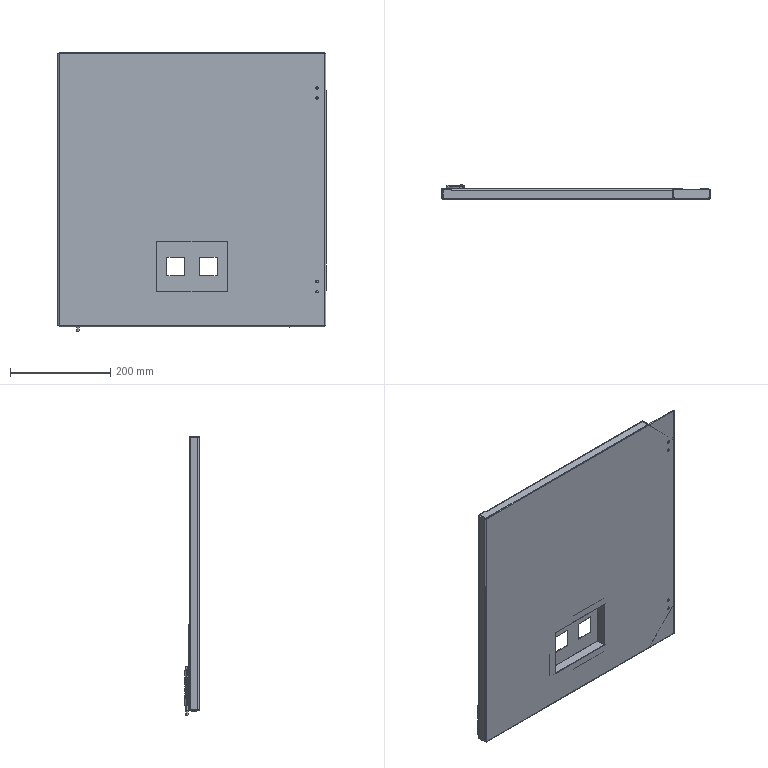Part | NX | features BREP 7 | 8 solids | 230 faces | box 534.5 x 29.2 x 557.003 mm | volume 569725 mm3 | plane 150 | cylinder 66 | torus 8 | spline 4 | cone 2 | commonest cylinder face diameters 6 x16 3 x12 5 x8 10 x8 0.8 x7 4 x6